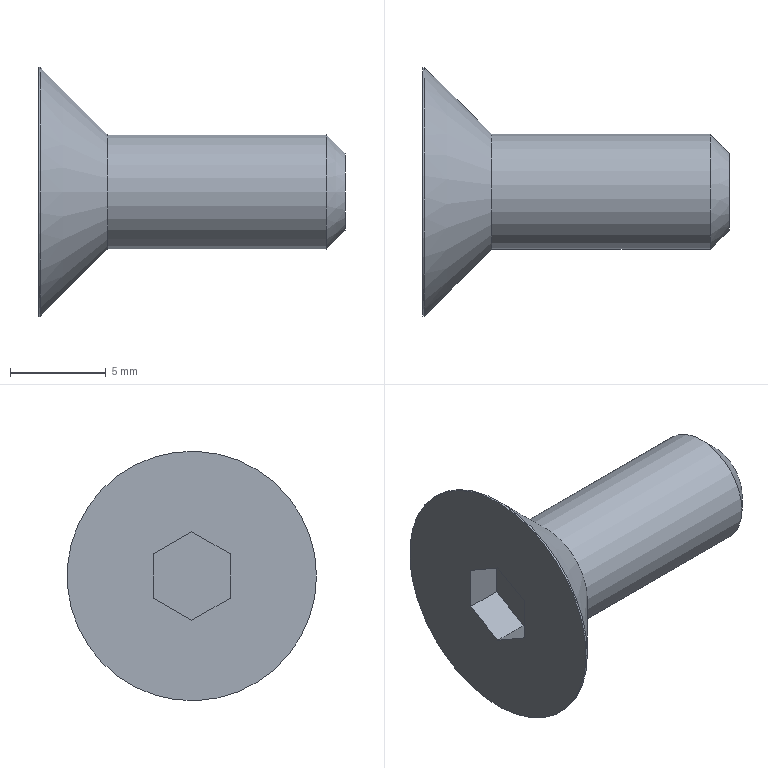Part | NX | features 5003_343_C-SFB6-16(Default) 2 | 1 solid | 13 faces | box 16 x 13 x 13 mm | volume 588.483 mm3 | plane 9 | cylinder 2 | cone 2 | commonest cylinder face diameters 6 x1 13 x1
STEP:
#1=CARTESIAN_POINT('',(200.825,88.9,-47.));
#2=VERTEX_POINT('',#1);
#3=CARTESIAN_POINT('',(200.825,85.9,-47.));
#4=DIRECTION('',(1.,0.,0.));
#5=DIRECTION('',(0.,1.,0.));
#6=AXIS2_PLACEMENT_3D('',#3,#4,#5);
#7=CIRCLE('',#6,3.);
#8=EDGE_CURVE('',#2,#2,#7,.F.);
#9=ORIENTED_EDGE('',*,*,#8,.T.);
#10=EDGE_LOOP('',(#9));
#11=FACE_BOUND('',#10,.T.);
#12=CARTESIAN_POINT('',(189.425,82.9,-47.));
#13=VERTEX_POINT('',#12);
#14=CARTESIAN_POINT('',(189.425,85.9,-47.));
#15=DIRECTION('',(-1.,0.,0.));
#16=DIRECTION('',(0.,-1.,0.));
#17=AXIS2_PLACEMENT_3D('',#14,#15,#16);
#18=CIRCLE('',#17,3.);
#19=EDGE_CURVE('',#13,#13,#18,.T.);
#20=ORIENTED_EDGE('',*,*,#19,.F.);
#21=EDGE_LOOP('',(#20));
#22=FACE_BOUND('',#21,.T.);
#23=CARTESIAN_POINT('',(185.825,85.9,-47.));
#24=DIRECTION('',(-1.,0.,0.));
#25=DIRECTION('',(0.,-1.,0.));
#26=AXIS2_PLACEMENT_3D('',#23,#24,#25);
#27=CYLINDRICAL_SURFACE('',#26,3.);
#28=ADVANCED_FACE('',(#11,#22),#27,.T.);
#29=CARTESIAN_POINT('',(185.825,83.9,-45.845));
#30=VERTEX_POINT('',#29);
#31=CARTESIAN_POINT('',(185.825,85.9,-44.691));
#32=VERTEX_POINT('',#31);
#33=CARTESIAN_POINT('',(185.825,83.9,-45.845));
#34=DIRECTION('',(0.,0.866,0.5));
#35=VECTOR('',#34,1000.);
#36=LINE('',#33,#35);
#37=EDGE_CURVE('',#30,#32,#36,.T.);
#38=ORIENTED_EDGE('',*,*,#37,.F.);
#39=CARTESIAN_POINT('',(185.825,83.9,-48.155));
#40=VERTEX_POINT('',#39);
#41=CARTESIAN_POINT('',(185.825,83.9,-48.155));
#42=DIRECTION('',(0.,0.,1.));
#43=VECTOR('',#42,1000.);
#44=LINE('',#41,#43);
#45=EDGE_CURVE('',#40,#30,#44,.T.);
#46=ORIENTED_EDGE('',*,*,#45,.F.);
#47=CARTESIAN_POINT('',(185.825,85.9,-49.309));
#48=VERTEX_POINT('',#47);
#49=CARTESIAN_POINT('',(185.825,85.9,-49.309));
#50=DIRECTION('',(0.,-0.866,0.5));
#51=VECTOR('',#50,1000.);
#52=LINE('',#49,#51);
#53=EDGE_CURVE('',#48,#40,#52,.T.);
#54=ORIENTED_EDGE('',*,*,#53,.F.);
#55=CARTESIAN_POINT('',(185.825,87.9,-48.155));
#56=VERTEX_POINT('',#55);
#57=CARTESIAN_POINT('',(185.825,87.9,-48.155));
#58=DIRECTION('',(0.,-0.866,-0.5));
#59=VECTOR('',#58,1000.);
#60=LINE('',#57,#59);
#61=EDGE_CURVE('',#56,#48,#60,.T.);
#62=ORIENTED_EDGE('',*,*,#61,.F.);
#63=CARTESIAN_POINT('',(185.825,87.9,-45.845));
#64=VERTEX_POINT('',#63);
#65=CARTESIAN_POINT('',(185.825,87.9,-45.845));
#66=DIRECTION('',(0.,0.,-1.));
#67=VECTOR('',#66,1000.);
#68=LINE('',#65,#67);
#69=EDGE_CURVE('',#64,#56,#68,.T.);
#70=ORIENTED_EDGE('',*,*,#69,.F.);
#71=CARTESIAN_POINT('',(185.825,85.9,-44.691));
#72=DIRECTION('',(0.,0.866,-0.5));
#73=VECTOR('',#72,1000.);
#74=LINE('',#71,#73);
#75=EDGE_CURVE('',#32,#64,#74,.T.);
#76=ORIENTED_EDGE('',*,*,#75,.F.);
#77=EDGE_LOOP('',(#38,#46,#54,#62,#70,#76));
#78=FACE_BOUND('',#77,.T.);
#79=CARTESIAN_POINT('',(185.825,79.4,-47.));
#80=VERTEX_POINT('',#79);
#81=CARTESIAN_POINT('',(185.825,85.9,-47.));
#82=DIRECTION('',(-1.,0.,0.));
#83=DIRECTION('',(0.,-1.,0.));
#84=AXIS2_PLACEMENT_3D('',#81,#82,#83);
#85=CIRCLE('',#84,6.5);
#86=EDGE_CURVE('',#80,#80,#85,.T.);
#87=ORIENTED_EDGE('',*,*,#86,.T.);
#88=EDGE_LOOP('',(#87));
#89=FACE_BOUND('',#88,.T.);
#90=CARTESIAN_POINT('',(185.825,85.9,-53.5));
#91=DIRECTION('',(-1.,0.,0.));
#92=DIRECTION('',(0.,-1.,0.));
#93=AXIS2_PLACEMENT_3D('',#90,#91,#92);
#94=PLANE('',#93);
#95=ADVANCED_FACE('',(#78,#89),#94,.T.);
#96=CARTESIAN_POINT('',(185.925,79.4,-47.));
#97=VERTEX_POINT('',#96);
#98=CARTESIAN_POINT('',(185.925,85.9,-47.));
#99=DIRECTION('',(-1.,0.,0.));
#100=DIRECTION('',(0.,-1.,0.));
#101=AXIS2_PLACEMENT_3D('',#98,#99,#100);
#102=CIRCLE('',#101,6.5);
#103=EDGE_CURVE('',#97,#97,#102,.T.);
#104=ORIENTED_EDGE('',*,*,#103,.T.);
#105=EDGE_LOOP('',(#104));
#106=FACE_BOUND('',#105,.T.);
#107=ORIENTED_EDGE('',*,*,#86,.F.);
#108=EDGE_LOOP('',(#107));
#109=FACE_BOUND('',#108,.T.);
#110=CARTESIAN_POINT('',(185.825,85.9,-47.));
#111=DIRECTION('',(-1.,0.,0.));
#112=DIRECTION('',(0.,-1.,0.));
#113=AXIS2_PLACEMENT_3D('',#110,#111,#112);
#114=CYLINDRICAL_SURFACE('',#113,6.5);
#115=ADVANCED_FACE('',(#106,#109),#114,.T.);
#116=ORIENTED_EDGE('',*,*,#19,.T.);
#117=EDGE_LOOP('',(#116));
#118=FACE_BOUND('',#117,.T.);
#119=ORIENTED_EDGE('',*,*,#103,.F.);
#120=EDGE_LOOP('',(#119));
#121=FACE_BOUND('',#120,.T.);
#122=CARTESIAN_POINT('',(185.925,85.9,-47.));
#123=DIRECTION('',(-1.,0.,0.));
#124=DIRECTION('',(0.,-1.,0.));
#125=AXIS2_PLACEMENT_3D('',#122,#123,#124);
#126=CONICAL_SURFACE('',#125,6.5,0.7854);
#127=ADVANCED_FACE('',(#118,#121),#126,.T.);
#128=ORIENTED_EDGE('',*,*,#37,.T.);
#129=CARTESIAN_POINT('',(187.725,85.9,-44.691));
#130=VERTEX_POINT('',#129);
#131=CARTESIAN_POINT('',(187.725,85.9,-44.691));
#132=DIRECTION('',(-1.,0.,0.));
#133=VECTOR('',#132,1000.);
#134=LINE('',#131,#133);
#135=EDGE_CURVE('',#130,#32,#134,.T.);
#136=ORIENTED_EDGE('',*,*,#135,.F.);
#137=CARTESIAN_POINT('',(187.725,83.9,-45.845));
#138=VERTEX_POINT('',#137);
#139=CARTESIAN_POINT('',(187.725,83.9,-45.845));
#140=DIRECTION('',(0.,0.866,0.5));
#141=VECTOR('',#140,1000.);
#142=LINE('',#139,#141);
#143=EDGE_CURVE('',#138,#130,#142,.T.);
#144=ORIENTED_EDGE('',*,*,#143,.F.);
#145=CARTESIAN_POINT('',(187.725,83.9,-45.845));
#146=DIRECTION('',(-1.,0.,0.));
#147=VECTOR('',#146,1000.);
#148=LINE('',#145,#147);
#149=EDGE_CURVE('',#138,#30,#148,.T.);
#150=ORIENTED_EDGE('',*,*,#149,.T.);
#151=EDGE_LOOP('',(#128,#136,#144,#150));
#152=FACE_BOUND('',#151,.T.);
#153=CARTESIAN_POINT('',(187.725,83.9,-45.845));
#154=DIRECTION('',(0.,-0.5,0.866));
#155=DIRECTION('',(0.,-0.866,-0.5));
#156=AXIS2_PLACEMENT_3D('',#153,#154,#155);
#157=PLANE('',#156);
#158=ADVANCED_FACE('',(#152),#157,.F.);
#159=ORIENTED_EDGE('',*,*,#45,.T.);
#160=ORIENTED_EDGE('',*,*,#149,.F.);
#161=CARTESIAN_POINT('',(187.725,83.9,-48.155));
#162=VERTEX_POINT('',#161);
#163=CARTESIAN_POINT('',(187.725,83.9,-48.155));
#164=DIRECTION('',(0.,0.,1.));
#165=VECTOR('',#164,1000.);
#166=LINE('',#163,#165);
#167=EDGE_CURVE('',#162,#138,#166,.T.);
#168=ORIENTED_EDGE('',*,*,#167,.F.);
#169=CARTESIAN_POINT('',(187.725,83.9,-48.155));
#170=DIRECTION('',(-1.,0.,0.));
#171=VECTOR('',#170,1000.);
#172=LINE('',#169,#171);
#173=EDGE_CURVE('',#162,#40,#172,.T.);
#174=ORIENTED_EDGE('',*,*,#173,.T.);
#175=EDGE_LOOP('',(#159,#160,#168,#174));
#176=FACE_BOUND('',#175,.T.);
#177=CARTESIAN_POINT('',(187.725,83.9,-48.155));
#178=DIRECTION('',(0.,-1.,0.));
#179=DIRECTION('',(1.,0.,0.));
#180=AXIS2_PLACEMENT_3D('',#177,#178,#179);
#181=PLANE('',#180);
#182=ADVANCED_FACE('',(#176),#181,.F.);
#183=ORIENTED_EDGE('',*,*,#53,.T.);
#184=ORIENTED_EDGE('',*,*,#173,.F.);
#185=CARTESIAN_POINT('',(187.725,85.9,-49.309));
#186=VERTEX_POINT('',#185);
#187=CARTESIAN_POINT('',(187.725,85.9,-49.309));
#188=DIRECTION('',(0.,-0.866,0.5));
#189=VECTOR('',#188,1000.);
#190=LINE('',#187,#189);
#191=EDGE_CURVE('',#186,#162,#190,.T.);
#192=ORIENTED_EDGE('',*,*,#191,.F.);
#193=CARTESIAN_POINT('',(187.725,85.9,-49.309));
#194=DIRECTION('',(-1.,0.,0.));
#195=VECTOR('',#194,1000.);
#196=LINE('',#193,#195);
#197=EDGE_CURVE('',#186,#48,#196,.T.);
#198=ORIENTED_EDGE('',*,*,#197,.T.);
#199=EDGE_LOOP('',(#183,#184,#192,#198));
#200=FACE_BOUND('',#199,.T.);
#201=CARTESIAN_POINT('',(187.725,85.9,-49.309));
#202=DIRECTION('',(0.,-0.5,-0.866));
#203=DIRECTION('',(0.,0.866,-0.5));
#204=AXIS2_PLACEMENT_3D('',#201,#202,#203);
#205=PLANE('',#204);
#206=ADVANCED_FACE('',(#200),#205,.F.);
#207=ORIENTED_EDGE('',*,*,#61,.T.);
#208=ORIENTED_EDGE('',*,*,#197,.F.);
#209=CARTESIAN_POINT('',(187.725,87.9,-48.155));
#210=VERTEX_POINT('',#209);
#211=CARTESIAN_POINT('',(187.725,87.9,-48.155));
#212=DIRECTION('',(0.,-0.866,-0.5));
#213=VECTOR('',#212,1000.);
#214=LINE('',#211,#213);
#215=EDGE_CURVE('',#210,#186,#214,.T.);
#216=ORIENTED_EDGE('',*,*,#215,.F.);
#217=CARTESIAN_POINT('',(187.725,87.9,-48.155));
#218=DIRECTION('',(-1.,0.,0.));
#219=VECTOR('',#218,1000.);
#220=LINE('',#217,#219);
#221=EDGE_CURVE('',#210,#56,#220,.T.);
#222=ORIENTED_EDGE('',*,*,#221,.T.);
#223=EDGE_LOOP('',(#207,#208,#216,#222));
#224=FACE_BOUND('',#223,.T.);
#225=CARTESIAN_POINT('',(187.725,87.9,-48.155));
#226=DIRECTION('',(0.,0.5,-0.866));
#227=DIRECTION('',(0.,0.866,0.5));
#228=AXIS2_PLACEMENT_3D('',#225,#226,#227);
#229=PLANE('',#228);
#230=ADVANCED_FACE('',(#224),#229,.F.);
#231=ORIENTED_EDGE('',*,*,#69,.T.);
#232=ORIENTED_EDGE('',*,*,#221,.F.);
#233=CARTESIAN_POINT('',(187.725,87.9,-45.845));
#234=VERTEX_POINT('',#233);
#235=CARTESIAN_POINT('',(187.725,87.9,-45.845));
#236=DIRECTION('',(0.,0.,-1.));
#237=VECTOR('',#236,1000.);
#238=LINE('',#235,#237);
#239=EDGE_CURVE('',#234,#210,#238,.T.);
#240=ORIENTED_EDGE('',*,*,#239,.F.);
#241=CARTESIAN_POINT('',(187.725,87.9,-45.845));
#242=DIRECTION('',(-1.,0.,0.));
#243=VECTOR('',#242,1000.);
#244=LINE('',#241,#243);
#245=EDGE_CURVE('',#234,#64,#244,.T.);
#246=ORIENTED_EDGE('',*,*,#245,.T.);
#247=EDGE_LOOP('',(#231,#232,#240,#246));
#248=FACE_BOUND('',#247,.T.);
#249=CARTESIAN_POINT('',(187.725,87.9,-45.845));
#250=DIRECTION('',(0.,1.,0.));
#251=DIRECTION('',(-1.,0.,0.));
#252=AXIS2_PLACEMENT_3D('',#249,#250,#251);
#253=PLANE('',#252);
#254=ADVANCED_FACE('',(#248),#253,.F.);
#255=ORIENTED_EDGE('',*,*,#75,.T.);
#256=ORIENTED_EDGE('',*,*,#245,.F.);
#257=CARTESIAN_POINT('',(187.725,85.9,-44.691));
#258=DIRECTION('',(0.,0.866,-0.5));
#259=VECTOR('',#258,1000.);
#260=LINE('',#257,#259);
#261=EDGE_CURVE('',#130,#234,#260,.T.);
#262=ORIENTED_EDGE('',*,*,#261,.F.);
#263=ORIENTED_EDGE('',*,*,#135,.T.);
#264=EDGE_LOOP('',(#255,#256,#262,#263));
#265=FACE_BOUND('',#264,.T.);
#266=CARTESIAN_POINT('',(187.725,85.9,-44.691));
#267=DIRECTION('',(0.,0.5,0.866));
#268=DIRECTION('',(0.,-0.866,0.5));
#269=AXIS2_PLACEMENT_3D('',#266,#267,#268);
#270=PLANE('',#269);
#271=ADVANCED_FACE('',(#265),#270,.F.);
#272=ORIENTED_EDGE('',*,*,#143,.T.);
#273=ORIENTED_EDGE('',*,*,#261,.T.);
#274=ORIENTED_EDGE('',*,*,#239,.T.);
#275=ORIENTED_EDGE('',*,*,#215,.T.);
#276=ORIENTED_EDGE('',*,*,#191,.T.);
#277=ORIENTED_EDGE('',*,*,#167,.T.);
#278=EDGE_LOOP('',(#272,#273,#274,#275,#276,#277));
#279=FACE_BOUND('',#278,.T.);
#280=CARTESIAN_POINT('',(187.725,85.9,-47.));
#281=DIRECTION('',(-1.,0.,0.));
#282=DIRECTION('',(0.,-1.,0.));
#283=AXIS2_PLACEMENT_3D('',#280,#281,#282);
#284=PLANE('',#283);
#285=ADVANCED_FACE('',(#279),#284,.T.);
#286=CARTESIAN_POINT('',(201.825,87.9,-47.));
#287=VERTEX_POINT('',#286);
#288=CARTESIAN_POINT('',(201.825,85.9,-47.));
#289=DIRECTION('',(1.,0.,0.));
#290=DIRECTION('',(0.,1.,0.));
#291=AXIS2_PLACEMENT_3D('',#288,#289,#290);
#292=CIRCLE('',#291,2.);
#293=EDGE_CURVE('',#287,#287,#292,.T.);
#294=ORIENTED_EDGE('',*,*,#293,.T.);
#295=EDGE_LOOP('',(#294));
#296=FACE_BOUND('',#295,.T.);
#297=CARTESIAN_POINT('',(201.825,75.9,-43.));
#298=DIRECTION('',(1.,0.,0.));
#299=DIRECTION('',(0.,1.,0.));
#300=AXIS2_PLACEMENT_3D('',#297,#298,#299);
#301=PLANE('',#300);
#302=ADVANCED_FACE('',(#296),#301,.T.);
#303=ORIENTED_EDGE('',*,*,#293,.F.);
#304=EDGE_LOOP('',(#303));
#305=FACE_BOUND('',#304,.T.);
#306=ORIENTED_EDGE('',*,*,#8,.F.);
#307=EDGE_LOOP('',(#306));
#308=FACE_BOUND('',#307,.T.);
#309=CARTESIAN_POINT('',(200.825,85.9,-47.));
#310=DIRECTION('',(-1.,0.,0.));
#311=DIRECTION('',(0.,-1.,0.));
#312=AXIS2_PLACEMENT_3D('',#309,#310,#311);
#313=CONICAL_SURFACE('',#312,3.,0.7854);
#314=ADVANCED_FACE('',(#305,#308),#313,.T.);
#315=CLOSED_SHELL('',(#28,#95,#115,#127,#158,#182,#206,#230,#254,#271,#285,#302,#314));
#316=MANIFOLD_SOLID_BREP('',#315);
#317=(LENGTH_UNIT()NAMED_UNIT(*)SI_UNIT(.MILLI.,.METRE.));
#318=UNCERTAINTY_MEASURE_WITH_UNIT(LENGTH_MEASURE(0.00001),#317,'','');
#319=(NAMED_UNIT(*)PLANE_ANGLE_UNIT()SI_UNIT($,.RADIAN.));
#320=(NAMED_UNIT(*)SI_UNIT($,.STERADIAN.)SOLID_ANGLE_UNIT());
#321=(GEOMETRIC_REPRESENTATION_CONTEXT(3)GLOBAL_UNCERTAINTY_ASSIGNED_CONTEXT((#318))GLOBAL_UNIT_ASSIGNED_CONTEXT((#317,#319,#320))REPRESENTATION_CONTEXT('',''));
#322=ADVANCED_BREP_SHAPE_REPRESENTATION('',(#316),#321);